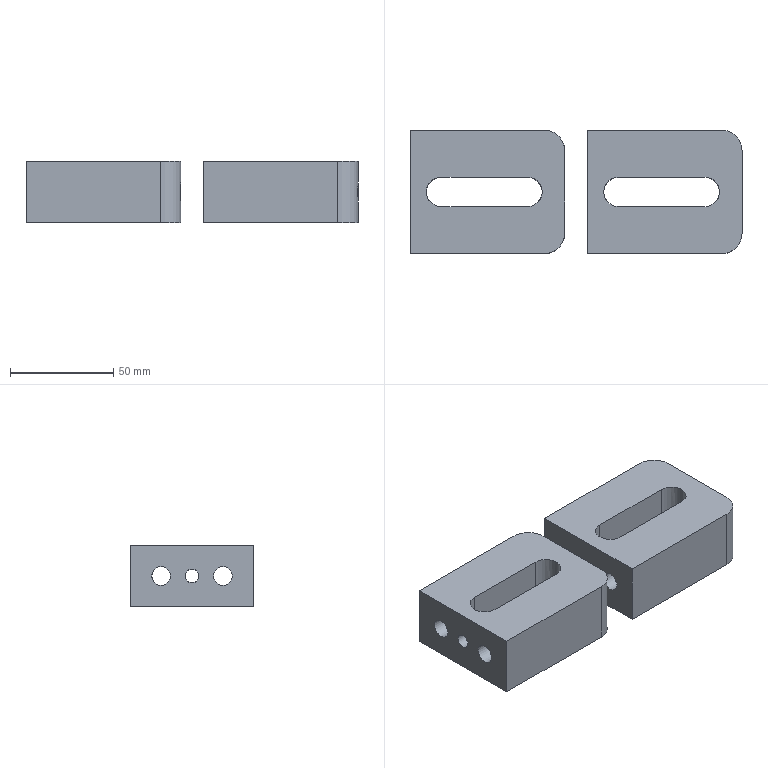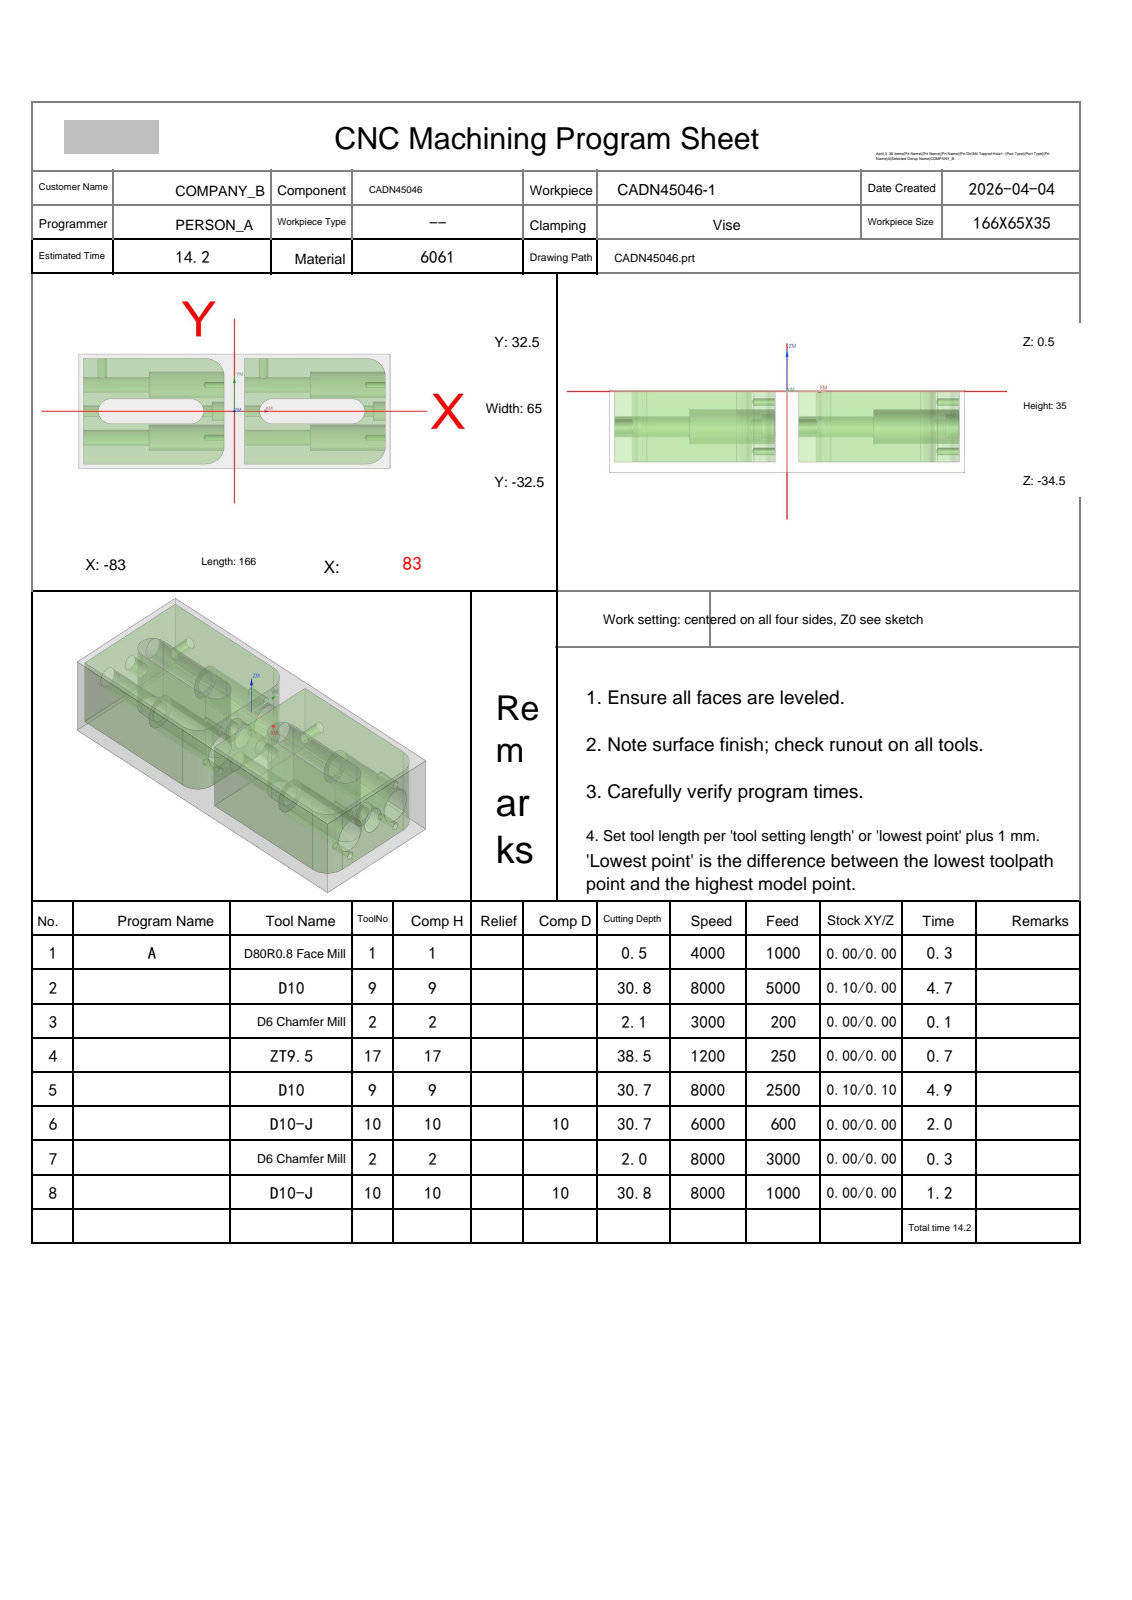NC program | NX | posted by the shop | part box 161 x 60 x 30 mm
Whole program, first 1260 of 1901 lines:
%
O0001
(Machine time: 15.73 MIN)
(===Total Tool:5===)
(T1=D80R0.8 Face Mill D=80.  R=0.8  D-  H01 Z=0.    )
(T9=D10     D=10.  R=0.   D-  H09 Z=-30.3 )
(T2=D6 Chamfer Mill   D=6.   R=0.   D-  H02 Z=-1.55 )
(T17=ZT9.5  D=9.5  DR_a=118 D-  H17 Z=-38.  )
(T10=D10-J  D=10.  R=0.   D10 H10 Z=-30.3 )
G80 G90 G17 G49 G40
G91 G28 Z0
M01
N1 T01 M06
(D80R0.8 Face Mill  D=80. R=0.8 H=01 ce=0.00 di=0.00)
G00 G90 G54 X-125.5 Y0.0 M03 S4000
G43 H01 Z20.
M08
Z2.
G01 Z0.0 F1000.
X-120.5
X120.5
X125.5
Z2.
G00 Z20.
G91 G28 Z0.0
M05
M09
G91 G28 Z0.0
M01
N2 T09 M06
(D10  D=10. R=0. H=09 ce=0.10 di=0.00)
G00 G90 G54 X38. Y35.1 M03 S8000
G43 H09 Z20.
M08
Z.5
G01 X70.5 Z.413 F5000.
G02 X85.6 Y20. Z.349 I0.0 J-15.1
G01 Y-20. Z.241
G02 X70.5 Y-35.1 Z.177 I-15.1 J0.0
G01 X5.5 Z.002
G02 X.4 Y-30. Z-.019 I0.0 J5.1
G01 Y30. Z-.181
G02 X5.5 Y35.1 Z-.202 I5.1 J0.0
G01 X70.5 Z-.377
G02 X85.6 Y20. Z-.441 I0.0 J-15.1
G01 Y-20. Z-.549
G02 X70.5 Y-35.1 Z-.613 I-15.1 J0.0
G01 X5.5 Z-.787
G02 X.4 Y-30. Z-.809 I0.0 J5.1
G01 Y30. Z-.97
G02 X5.5 Y35.1 Z-.992 I5.1 J0.0
G01 X70.5 Z-1.167
G02 X85.6 Y20. Z-1.231 I0.0 J-15.1
G01 Y-20. Z-1.338
G02 X70.5 Y-35.1 Z-1.402 I-15.1 J0.0
G01 X5.5 Z-1.577
G02 X.4 Y-30. Z-1.599 I0.0 J5.1
G01 Y30. Z-1.76
G02 X5.5 Y35.1 Z-1.782 I5.1 J0.0
G01 X70.5 Z-1.957
G02 X85.6 Y20. Z-2.021 I0.0 J-15.1
G01 Y-20. Z-2.128
G02 X70.5 Y-35.1 Z-2.192 I-15.1 J0.0
G01 X5.5 Z-2.367
G02 X.4 Y-30. Z-2.388 I0.0 J5.1
G01 Y30. Z-2.55
G02 X5.5 Y35.1 Z-2.572 I5.1 J0.0
G01 X70.5 Z-2.746
G02 X85.6 Y20. Z-2.81 I0.0 J-15.1
G01 Y-20. Z-2.918
G02 X70.5 Y-35.1 Z-2.982 I-15.1 J0.0
G01 X5.5 Z-3.157
G02 X.4 Y-30. Z-3.178 I0.0 J5.1
G01 Y30. Z-3.34
G02 X5.5 Y35.1 Z-3.361 I5.1 J0.0
G01 X70.5 Z-3.536
G02 X85.6 Y20. Z-3.6 I0.0 J-15.1
G01 Y-20. Z-3.708
G02 X70.5 Y-35.1 Z-3.771 I-15.1 J0.0
G01 X5.5 Z-3.946
G02 X.4 Y-30. Z-3.968 I0.0 J5.1
G01 Y30. Z-4.129
G02 X5.5 Y35.1 Z-4.151 I5.1 J0.0
G01 X70.5 Z-4.326
G02 X85.6 Y20. Z-4.39 I0.0 J-15.1
G01 Y-20. Z-4.497
G02 X70.5 Y-35.1 Z-4.561 I-15.1 J0.0
G01 X5.5 Z-4.736
G02 X.4 Y-30. Z-4.758 I0.0 J5.1
G01 Y30. Z-4.919
G02 X5.5 Y35.1 Z-4.941 I5.1 J0.0
G01 X70.5 Z-5.116
G02 X85.6 Y20. Z-5.179 I0.0 J-15.1
G01 Y-20. Z-5.287
G02 X70.5 Y-35.1 Z-5.351 I-15.1 J0.0
G01 X5.5 Z-5.526
G02 X.4 Y-30. Z-5.547 I0.0 J5.1
G01 Y30. Z-5.709
G02 X5.5 Y35.1 Z-5.73 I5.1 J0.0
G01 X70.5 Z-5.905
G02 X85.6 Y20. Z-5.969 I0.0 J-15.1
G01 Y-20. Z-6.077
G02 X70.5 Y-35.1 Z-6.141 I-15.1 J0.0
G01 X5.5 Z-6.316
G02 X.4 Y-30. Z-6.337 I0.0 J5.1
G01 Y30. Z-6.499
G02 X5.5 Y35.1 Z-6.52 I5.1 J0.0
G01 X70.5 Z-6.695
G02 X85.6 Y20. Z-6.759 I0.0 J-15.1
G01 Y-20. Z-6.867
G02 X70.5 Y-35.1 Z-6.93 I-15.1 J0.0
G01 X5.5 Z-7.105
G02 X.4 Y-30. Z-7.127 I0.0 J5.1
G01 Y30. Z-7.288
G02 X5.5 Y35.1 Z-7.31 I5.1 J0.0
G01 X70.5 Z-7.485
G02 X85.6 Y20. Z-7.549 I0.0 J-15.1
G01 Y-20. Z-7.656
G02 X70.5 Y-35.1 Z-7.72 I-15.1 J0.0
G01 X5.5 Z-7.895
G02 X.4 Y-30. Z-7.917 I0.0 J5.1
G01 Y30. Z-8.078
G02 X5.5 Y35.1 Z-8.1 I5.1 J0.0
G01 X70.5 Z-8.275
G02 X85.6 Y20. Z-8.338 I0.0 J-15.1
G01 Y-20. Z-8.446
G02 X70.5 Y-35.1 Z-8.51 I-15.1 J0.0
G01 X5.5 Z-8.685
G02 X.4 Y-30. Z-8.706 I0.0 J5.1
G01 Y30. Z-8.868
G02 X5.5 Y35.1 Z-8.889 I5.1 J0.0
G01 X70.5 Z-9.064
G02 X85.6 Y20. Z-9.128 I0.0 J-15.1
G01 Y-20. Z-9.236
G02 X70.5 Y-35.1 Z-9.3 I-15.1 J0.0
G01 X5.5 Z-9.475
G02 X.4 Y-30. Z-9.496 I0.0 J5.1
G01 Y30. Z-9.658
G02 X5.5 Y35.1 Z-9.679 I5.1 J0.0
G01 X70.5 Z-9.854
G02 X85.6 Y20. Z-9.918 I0.0 J-15.1
G01 Y-20. Z-10.026
G02 X70.5 Y-35.1 Z-10.089 I-15.1 J0.0
G01 X5.5 Z-10.264
G02 X.4 Y-30. Z-10.286 I0.0 J5.1
G01 Y30. Z-10.447
G02 X5.5 Y35.1 Z-10.469 I5.1 J0.0
G01 X70.5 Z-10.644
G02 X85.6 Y20. Z-10.708 I0.0 J-15.1
G01 Y-20. Z-10.815
G02 X70.5 Y-35.1 Z-10.879 I-15.1 J0.0
G01 X5.5 Z-11.054
G02 X.4 Y-30. Z-11.076 I0.0 J5.1
G01 Y30. Z-11.237
G02 X5.5 Y35.1 Z-11.259 I5.1 J0.0
G01 X70.5 Z-11.434
G02 X85.6 Y20. Z-11.497 I0.0 J-15.1
G01 Y-20. Z-11.605
G02 X70.5 Y-35.1 Z-11.669 I-15.1 J0.0
G01 X5.5 Z-11.844
G02 X.4 Y-30. Z-11.865 I0.0 J5.1
G01 Y30. Z-12.027
G02 X5.5 Y35.1 Z-12.048 I5.1 J0.0
G01 X70.5 Z-12.223
G02 X85.6 Y20. Z-12.287 I0.0 J-15.1
G01 Y-20. Z-12.395
G02 X70.5 Y-35.1 Z-12.459 I-15.1 J0.0
G01 X5.5 Z-12.634
G02 X.4 Y-30. Z-12.655 I0.0 J5.1
G01 Y30. Z-12.817
G02 X5.5 Y35.1 Z-12.838 I5.1 J0.0
G01 X70.5 Z-13.013
G02 X85.6 Y20. Z-13.077 I0.0 J-15.1
G01 Y-20. Z-13.185
G02 X70.5 Y-35.1 Z-13.248 I-15.1 J0.0
G01 X5.5 Z-13.423
G02 X.4 Y-30. Z-13.445 I0.0 J5.1
G01 Y30. Z-13.606
G02 X5.5 Y35.1 Z-13.628 I5.1 J0.0
G01 X70.5 Z-13.803
G02 X85.6 Y20. Z-13.867 I0.0 J-15.1
G01 Y-20. Z-13.974
G02 X70.5 Y-35.1 Z-14.038 I-15.1 J0.0
G01 X5.5 Z-14.213
G02 X.4 Y-30. Z-14.235 I0.0 J5.1
G01 Y30. Z-14.396
G02 X5.5 Y35.1 Z-14.418 I5.1 J0.0
G01 X70.5 Z-14.593
G02 X85.6 Y20. Z-14.656 I0.0 J-15.1
G01 Y-20. Z-14.764
G02 X70.5 Y-35.1 Z-14.828 I-15.1 J0.0
G01 X5.5 Z-15.003
G02 X.4 Y-30. Z-15.024 I0.0 J5.1
G01 Y30. Z-15.186
G02 X5.5 Y35.1 Z-15.207 I5.1 J0.0
G01 X70.5 Z-15.382
G02 X85.6 Y20. Z-15.446 I0.0 J-15.1
G01 Y-20. Z-15.554
G02 X70.5 Y-35.1 Z-15.618 I-15.1 J0.0
G01 X5.5 Z-15.793
G02 X.4 Y-30. Z-15.814 I0.0 J5.1
G01 Y30. Z-15.976
G02 X5.5 Y35.1 Z-15.997 I5.1 J0.0
G01 X70.5 Z-16.172
G02 X85.6 Y20. Z-16.236 I0.0 J-15.1
G01 Y-20. Z-16.344
G02 X70.5 Y-35.1 Z-16.407 I-15.1 J0.0
G01 X5.5 Z-16.582
G02 X.4 Y-30. Z-16.604 I0.0 J5.1
G01 Y30. Z-16.765
G02 X5.5 Y35.1 Z-16.787 I5.1 J0.0
G01 X70.5 Z-16.962
G02 X85.6 Y20. Z-17.026 I0.0 J-15.1
G01 Y-20. Z-17.133
G02 X70.5 Y-35.1 Z-17.197 I-15.1 J0.0
G01 X5.5 Z-17.372
G02 X.4 Y-30. Z-17.394 I0.0 J5.1
G01 Y30. Z-17.555
G02 X5.5 Y35.1 Z-17.577 I5.1 J0.0
G01 X70.5 Z-17.752
G02 X85.6 Y20. Z-17.815 I0.0 J-15.1
G01 Y-20. Z-17.923
G02 X70.5 Y-35.1 Z-17.987 I-15.1 J0.0
G01 X5.5 Z-18.162
G02 X.4 Y-30. Z-18.183 I0.0 J5.1
G01 Y30. Z-18.345
G02 X5.5 Y35.1 Z-18.366 I5.1 J0.0
G01 X70.5 Z-18.541
G02 X85.6 Y20. Z-18.605 I0.0 J-15.1
G01 Y-20. Z-18.713
G02 X70.5 Y-35.1 Z-18.777 I-15.1 J0.0
G01 X5.5 Z-18.952
G02 X.4 Y-30. Z-18.973 I0.0 J5.1
G01 Y30. Z-19.135
G02 X5.5 Y35.1 Z-19.156 I5.1 J0.0
G01 X70.5 Z-19.331
G02 X85.6 Y20. Z-19.395 I0.0 J-15.1
G01 Y-20. Z-19.503
G02 X70.5 Y-35.1 Z-19.566 I-15.1 J0.0
G01 X5.5 Z-19.741
G02 X.4 Y-30. Z-19.763 I0.0 J5.1
G01 Y30. Z-19.924
G02 X5.5 Y35.1 Z-19.946 I5.1 J0.0
G01 X70.5 Z-20.121
G02 X85.6 Y20. Z-20.185 I0.0 J-15.1
G01 Y-20. Z-20.292
G02 X70.5 Y-35.1 Z-20.356 I-15.1 J0.0
G01 X5.5 Z-20.531
G02 X.4 Y-30. Z-20.553 I0.0 J5.1
G01 Y30. Z-20.714
G02 X5.5 Y35.1 Z-20.736 I5.1 J0.0
G01 X70.5 Z-20.911
G02 X85.6 Y20. Z-20.974 I0.0 J-15.1
G01 Y-20. Z-21.082
G02 X70.5 Y-35.1 Z-21.146 I-15.1 J0.0
G01 X5.5 Z-21.321
G02 X.4 Y-30. Z-21.342 I0.0 J5.1
G01 Y30. Z-21.504
G02 X5.5 Y35.1 Z-21.525 I5.1 J0.0
G01 X70.5 Z-21.7
G02 X85.6 Y20. Z-21.764 I0.0 J-15.1
G01 Y-20. Z-21.872
G02 X70.5 Y-35.1 Z-21.936 I-15.1 J0.0
G01 X5.5 Z-22.111
G02 X.4 Y-30. Z-22.132 I0.0 J5.1
G01 Y30. Z-22.294
G02 X5.5 Y35.1 Z-22.315 I5.1 J0.0
G01 X70.5 Z-22.49
G02 X85.6 Y20. Z-22.554 I0.0 J-15.1
G01 Y-20. Z-22.662
G02 X70.5 Y-35.1 Z-22.725 I-15.1 J0.0
G01 X5.5 Z-22.9
G02 X.4 Y-30. Z-22.922 I0.0 J5.1
G01 Y30. Z-23.083
G02 X5.5 Y35.1 Z-23.105 I5.1 J0.0
G01 X70.5 Z-23.28
G02 X85.6 Y20. Z-23.344 I0.0 J-15.1
G01 Y-20. Z-23.451
G02 X70.5 Y-35.1 Z-23.515 I-15.1 J0.0
G01 X5.5 Z-23.69
G02 X.4 Y-30. Z-23.712 I0.0 J5.1
G01 Y30. Z-23.873
G02 X5.5 Y35.1 Z-23.895 I5.1 J0.0
G01 X70.5 Z-24.07
G02 X85.6 Y20. Z-24.133 I0.0 J-15.1
G01 Y-20. Z-24.241
G02 X70.5 Y-35.1 Z-24.305 I-15.1 J0.0
G01 X5.5 Z-24.48
G02 X.4 Y-30. Z-24.501 I0.0 J5.1
G01 Y30. Z-24.663
G02 X5.5 Y35.1 Z-24.684 I5.1 J0.0
G01 X70.5 Z-24.859
G02 X85.6 Y20. Z-24.923 I0.0 J-15.1
G01 Y-20. Z-25.031
G02 X70.5 Y-35.1 Z-25.095 I-15.1 J0.0
G01 X5.5 Z-25.269
G02 X.4 Y-30. Z-25.291 I0.0 J5.1
G01 Y30. Z-25.453
G02 X5.5 Y35.1 Z-25.474 I5.1 J0.0
G01 X70.5 Z-25.649
G02 X85.6 Y20. Z-25.713 I0.0 J-15.1
G01 Y-20. Z-25.82
G02 X70.5 Y-35.1 Z-25.884 I-15.1 J0.0
G01 X5.5 Z-26.059
G02 X.4 Y-30. Z-26.081 I0.0 J5.1
G01 Y30. Z-26.242
G02 X5.5 Y35.1 Z-26.264 I5.1 J0.0
G01 X70.5 Z-26.439
G02 X85.6 Y20. Z-26.503 I0.0 J-15.1
G01 Y-20. Z-26.61
G02 X70.5 Y-35.1 Z-26.674 I-15.1 J0.0
G01 X5.5 Z-26.849
G02 X.4 Y-30. Z-26.871 I0.0 J5.1
G01 Y30. Z-27.032
G02 X5.5 Y35.1 Z-27.054 I5.1 J0.0
G01 X70.5 Z-27.228
G02 X85.6 Y20. Z-27.292 I0.0 J-15.1
G01 Y-20. Z-27.4
G02 X70.5 Y-35.1 Z-27.464 I-15.1 J0.0
G01 X5.5 Z-27.639
G02 X.4 Y-30. Z-27.66 I0.0 J5.1
G01 Y30. Z-27.822
G02 X5.5 Y35.1 Z-27.843 I5.1 J0.0
G01 X70.5 Z-28.018
G02 X85.6 Y20. Z-28.082 I0.0 J-15.1
G01 Y-20. Z-28.19
G02 X70.5 Y-35.1 Z-28.254 I-15.1 J0.0
G01 X5.5 Z-28.428
G02 X.4 Y-30. Z-28.45 I0.0 J5.1
G01 Y30. Z-28.611
G02 X5.5 Y35.1 Z-28.633 I5.1 J0.0
G01 X70.5 Z-28.808
G02 X85.6 Y20. Z-28.872 I0.0 J-15.1
G01 Y-20. Z-28.979
G02 X70.5 Y-35.1 Z-29.043 I-15.1 J0.0
G01 X5.5 Z-29.218
G02 X.4 Y-30. Z-29.24 I0.0 J5.1
G01 Y30. Z-29.401
G02 X5.5 Y35.1 Z-29.423 I5.1 J0.0
G01 X70.5 Z-29.598
G02 X85.6 Y20. Z-29.662 I0.0 J-15.1
G01 Y-20. Z-29.769
G02 X70.5 Y-35.1 Z-29.833 I-15.1 J0.0
G01 X5.5 Z-30.008
G02 X.4 Y-30. Z-30.03 I0.0 J5.1
G01 Y30. Z-30.191
G02 X5.5 Y35.1 Z-30.213 I5.1 J0.0
G01 X38. Z-30.3
X70.5
G02 X85.6 Y20. I0.0 J-15.1
G01 Y-20.
G02 X70.5 Y-35.1 I-15.1 J0.0
G01 X5.5
G02 X.4 Y-30. I0.0 J5.1
G01 Y30.
G02 X5.5 Y35.1 I5.1 J0.0
G01 X38.
X38.5
Z-29.3
G00 Z20.
X-48.
Z.5
G01 X-15.5 Z.413
G02 X-.4 Y20. Z.349 I0.0 J-15.1
G01 Y-20. Z.241
G02 X-15.5 Y-35.1 Z.177 I-15.1 J0.0
G01 X-80.5 Z.002
G02 X-85.6 Y-30. Z-.019 I0.0 J5.1
G01 Y30. Z-.181
G02 X-80.5 Y35.1 Z-.202 I5.1 J0.0
G01 X-15.5 Z-.377
G02 X-.4 Y20. Z-.441 I0.0 J-15.1
G01 Y-20. Z-.549
G02 X-15.5 Y-35.1 Z-.613 I-15.1 J0.0
G01 X-80.5 Z-.787
G02 X-85.6 Y-30. Z-.809 I0.0 J5.1
G01 Y30. Z-.97
G02 X-80.5 Y35.1 Z-.992 I5.1 J0.0
G01 X-15.5 Z-1.167
G02 X-.4 Y20. Z-1.231 I0.0 J-15.1
G01 Y-20. Z-1.338
G02 X-15.5 Y-35.1 Z-1.402 I-15.1 J0.0
G01 X-80.5 Z-1.577
G02 X-85.6 Y-30. Z-1.599 I0.0 J5.1
G01 Y30. Z-1.76
G02 X-80.5 Y35.1 Z-1.782 I5.1 J0.0
G01 X-15.5 Z-1.957
G02 X-.4 Y20. Z-2.021 I0.0 J-15.1
G01 Y-20. Z-2.128
G02 X-15.5 Y-35.1 Z-2.192 I-15.1 J0.0
G01 X-80.5 Z-2.367
G02 X-85.6 Y-30. Z-2.388 I0.0 J5.1
G01 Y30. Z-2.55
G02 X-80.5 Y35.1 Z-2.572 I5.1 J0.0
G01 X-15.5 Z-2.746
G02 X-.4 Y20. Z-2.81 I0.0 J-15.1
G01 Y-20. Z-2.918
G02 X-15.5 Y-35.1 Z-2.982 I-15.1 J0.0
G01 X-80.5 Z-3.157
G02 X-85.6 Y-30. Z-3.178 I0.0 J5.1
G01 Y30. Z-3.34
G02 X-80.5 Y35.1 Z-3.361 I5.1 J0.0
G01 X-15.5 Z-3.536
G02 X-.4 Y20. Z-3.6 I0.0 J-15.1
G01 Y-20. Z-3.708
G02 X-15.5 Y-35.1 Z-3.771 I-15.1 J0.0
G01 X-80.5 Z-3.946
G02 X-85.6 Y-30. Z-3.968 I0.0 J5.1
G01 Y30. Z-4.129
G02 X-80.5 Y35.1 Z-4.151 I5.1 J0.0
G01 X-15.5 Z-4.326
G02 X-.4 Y20. Z-4.39 I0.0 J-15.1
G01 Y-20. Z-4.497
G02 X-15.5 Y-35.1 Z-4.561 I-15.1 J0.0
G01 X-80.5 Z-4.736
G02 X-85.6 Y-30. Z-4.758 I0.0 J5.1
G01 Y30. Z-4.919
G02 X-80.5 Y35.1 Z-4.941 I5.1 J0.0
G01 X-15.5 Z-5.116
G02 X-.4 Y20. Z-5.179 I0.0 J-15.1
G01 Y-20. Z-5.287
G02 X-15.5 Y-35.1 Z-5.351 I-15.1 J0.0
G01 X-80.5 Z-5.526
G02 X-85.6 Y-30. Z-5.547 I0.0 J5.1
G01 Y30. Z-5.709
G02 X-80.5 Y35.1 Z-5.73 I5.1 J0.0
G01 X-15.5 Z-5.905
G02 X-.4 Y20. Z-5.969 I0.0 J-15.1
G01 Y-20. Z-6.077
G02 X-15.5 Y-35.1 Z-6.141 I-15.1 J0.0
G01 X-80.5 Z-6.316
G02 X-85.6 Y-30. Z-6.337 I0.0 J5.1
G01 Y30. Z-6.499
G02 X-80.5 Y35.1 Z-6.52 I5.1 J0.0
G01 X-15.5 Z-6.695
G02 X-.4 Y20. Z-6.759 I0.0 J-15.1
G01 Y-20. Z-6.867
G02 X-15.5 Y-35.1 Z-6.93 I-15.1 J0.0
G01 X-80.5 Z-7.105
G02 X-85.6 Y-30. Z-7.127 I0.0 J5.1
G01 Y30. Z-7.288
G02 X-80.5 Y35.1 Z-7.31 I5.1 J0.0
G01 X-15.5 Z-7.485
G02 X-.4 Y20. Z-7.549 I0.0 J-15.1
G01 Y-20. Z-7.656
G02 X-15.5 Y-35.1 Z-7.72 I-15.1 J0.0
G01 X-80.5 Z-7.895
G02 X-85.6 Y-30. Z-7.917 I0.0 J5.1
G01 Y30. Z-8.078
G02 X-80.5 Y35.1 Z-8.1 I5.1 J0.0
G01 X-15.5 Z-8.275
G02 X-.4 Y20. Z-8.338 I0.0 J-15.1
G01 Y-20. Z-8.446
G02 X-15.5 Y-35.1 Z-8.51 I-15.1 J0.0
G01 X-80.5 Z-8.685
G02 X-85.6 Y-30. Z-8.706 I0.0 J5.1
G01 Y30. Z-8.868
G02 X-80.5 Y35.1 Z-8.889 I5.1 J0.0
G01 X-15.5 Z-9.064
G02 X-.4 Y20. Z-9.128 I0.0 J-15.1
G01 Y-20. Z-9.236
G02 X-15.5 Y-35.1 Z-9.3 I-15.1 J0.0
G01 X-80.5 Z-9.475
G02 X-85.6 Y-30. Z-9.496 I0.0 J5.1
G01 Y30. Z-9.658
G02 X-80.5 Y35.1 Z-9.679 I5.1 J0.0
G01 X-15.5 Z-9.854
G02 X-.4 Y20. Z-9.918 I0.0 J-15.1
G01 Y-20. Z-10.026
G02 X-15.5 Y-35.1 Z-10.089 I-15.1 J0.0
G01 X-80.5 Z-10.264
G02 X-85.6 Y-30. Z-10.286 I0.0 J5.1
G01 Y30. Z-10.447
G02 X-80.5 Y35.1 Z-10.469 I5.1 J0.0
G01 X-15.5 Z-10.644
G02 X-.4 Y20. Z-10.708 I0.0 J-15.1
G01 Y-20. Z-10.815
G02 X-15.5 Y-35.1 Z-10.879 I-15.1 J0.0
G01 X-80.5 Z-11.054
G02 X-85.6 Y-30. Z-11.076 I0.0 J5.1
G01 Y30. Z-11.237
G02 X-80.5 Y35.1 Z-11.259 I5.1 J0.0
G01 X-15.5 Z-11.434
G02 X-.4 Y20. Z-11.497 I0.0 J-15.1
G01 Y-20. Z-11.605
G02 X-15.5 Y-35.1 Z-11.669 I-15.1 J0.0
G01 X-80.5 Z-11.844
G02 X-85.6 Y-30. Z-11.865 I0.0 J5.1
G01 Y30. Z-12.027
G02 X-80.5 Y35.1 Z-12.048 I5.1 J0.0
G01 X-15.5 Z-12.223
G02 X-.4 Y20. Z-12.287 I0.0 J-15.1
G01 Y-20. Z-12.395
G02 X-15.5 Y-35.1 Z-12.459 I-15.1 J0.0
G01 X-80.5 Z-12.634
G02 X-85.6 Y-30. Z-12.655 I0.0 J5.1
G01 Y30. Z-12.817
G02 X-80.5 Y35.1 Z-12.838 I5.1 J0.0
G01 X-15.5 Z-13.013
G02 X-.4 Y20. Z-13.077 I0.0 J-15.1
G01 Y-20. Z-13.185
G02 X-15.5 Y-35.1 Z-13.248 I-15.1 J0.0
G01 X-80.5 Z-13.423
G02 X-85.6 Y-30. Z-13.445 I0.0 J5.1
G01 Y30. Z-13.606
G02 X-80.5 Y35.1 Z-13.628 I5.1 J0.0
G01 X-15.5 Z-13.803
G02 X-.4 Y20. Z-13.867 I0.0 J-15.1
G01 Y-20. Z-13.974
G02 X-15.5 Y-35.1 Z-14.038 I-15.1 J0.0
G01 X-80.5 Z-14.213
G02 X-85.6 Y-30. Z-14.235 I0.0 J5.1
G01 Y30. Z-14.396
G02 X-80.5 Y35.1 Z-14.418 I5.1 J0.0
G01 X-15.5 Z-14.593
G02 X-.4 Y20. Z-14.656 I0.0 J-15.1
G01 Y-20. Z-14.764
G02 X-15.5 Y-35.1 Z-14.828 I-15.1 J0.0
G01 X-80.5 Z-15.003
G02 X-85.6 Y-30. Z-15.024 I0.0 J5.1
G01 Y30. Z-15.186
G02 X-80.5 Y35.1 Z-15.207 I5.1 J0.0
G01 X-15.5 Z-15.382
G02 X-.4 Y20. Z-15.446 I0.0 J-15.1
G01 Y-20. Z-15.554
G02 X-15.5 Y-35.1 Z-15.618 I-15.1 J0.0
G01 X-80.5 Z-15.793
G02 X-85.6 Y-30. Z-15.814 I0.0 J5.1
G01 Y30. Z-15.976
G02 X-80.5 Y35.1 Z-15.997 I5.1 J0.0
G01 X-15.5 Z-16.172
G02 X-.4 Y20. Z-16.236 I0.0 J-15.1
G01 Y-20. Z-16.344
G02 X-15.5 Y-35.1 Z-16.407 I-15.1 J0.0
G01 X-80.5 Z-16.582
G02 X-85.6 Y-30. Z-16.604 I0.0 J5.1
G01 Y30. Z-16.765
G02 X-80.5 Y35.1 Z-16.787 I5.1 J0.0
G01 X-15.5 Z-16.962
G02 X-.4 Y20. Z-17.026 I0.0 J-15.1
G01 Y-20. Z-17.133
G02 X-15.5 Y-35.1 Z-17.197 I-15.1 J0.0
G01 X-80.5 Z-17.372
G02 X-85.6 Y-30. Z-17.394 I0.0 J5.1
G01 Y30. Z-17.555
G02 X-80.5 Y35.1 Z-17.577 I5.1 J0.0
G01 X-15.5 Z-17.752
G02 X-.4 Y20. Z-17.815 I0.0 J-15.1
G01 Y-20. Z-17.923
G02 X-15.5 Y-35.1 Z-17.987 I-15.1 J0.0
G01 X-80.5 Z-18.162
G02 X-85.6 Y-30. Z-18.183 I0.0 J5.1
G01 Y30. Z-18.345
G02 X-80.5 Y35.1 Z-18.366 I5.1 J0.0
G01 X-15.5 Z-18.541
G02 X-.4 Y20. Z-18.605 I0.0 J-15.1
G01 Y-20. Z-18.713
G02 X-15.5 Y-35.1 Z-18.777 I-15.1 J0.0
G01 X-80.5 Z-18.952
G02 X-85.6 Y-30. Z-18.973 I0.0 J5.1
G01 Y30. Z-19.135
G02 X-80.5 Y35.1 Z-19.156 I5.1 J0.0
G01 X-15.5 Z-19.331
G02 X-.4 Y20. Z-19.395 I0.0 J-15.1
G01 Y-20. Z-19.503
G02 X-15.5 Y-35.1 Z-19.566 I-15.1 J0.0
G01 X-80.5 Z-19.741
G02 X-85.6 Y-30. Z-19.763 I0.0 J5.1
G01 Y30. Z-19.924
G02 X-80.5 Y35.1 Z-19.946 I5.1 J0.0
G01 X-15.5 Z-20.121
G02 X-.4 Y20. Z-20.185 I0.0 J-15.1
G01 Y-20. Z-20.292
G02 X-15.5 Y-35.1 Z-20.356 I-15.1 J0.0
G01 X-80.5 Z-20.531
G02 X-85.6 Y-30. Z-20.553 I0.0 J5.1
G01 Y30. Z-20.714
G02 X-80.5 Y35.1 Z-20.736 I5.1 J0.0
G01 X-15.5 Z-20.911
G02 X-.4 Y20. Z-20.974 I0.0 J-15.1
G01 Y-20. Z-21.082
G02 X-15.5 Y-35.1 Z-21.146 I-15.1 J0.0
G01 X-80.5 Z-21.321
G02 X-85.6 Y-30. Z-21.342 I0.0 J5.1
G01 Y30. Z-21.504
G02 X-80.5 Y35.1 Z-21.525 I5.1 J0.0
G01 X-15.5 Z-21.7
G02 X-.4 Y20. Z-21.764 I0.0 J-15.1
G01 Y-20. Z-21.872
G02 X-15.5 Y-35.1 Z-21.936 I-15.1 J0.0
G01 X-80.5 Z-22.111
G02 X-85.6 Y-30. Z-22.132 I0.0 J5.1
G01 Y30. Z-22.294
G02 X-80.5 Y35.1 Z-22.315 I5.1 J0.0
G01 X-15.5 Z-22.49
G02 X-.4 Y20. Z-22.554 I0.0 J-15.1
G01 Y-20. Z-22.662
G02 X-15.5 Y-35.1 Z-22.725 I-15.1 J0.0
G01 X-80.5 Z-22.9
G02 X-85.6 Y-30. Z-22.922 I0.0 J5.1
G01 Y30. Z-23.083
G02 X-80.5 Y35.1 Z-23.105 I5.1 J0.0
G01 X-15.5 Z-23.28
G02 X-.4 Y20. Z-23.344 I0.0 J-15.1
G01 Y-20. Z-23.451
G02 X-15.5 Y-35.1 Z-23.515 I-15.1 J0.0
G01 X-80.5 Z-23.69
G02 X-85.6 Y-30. Z-23.712 I0.0 J5.1
G01 Y30. Z-23.873
G02 X-80.5 Y35.1 Z-23.895 I5.1 J0.0
G01 X-15.5 Z-24.07
G02 X-.4 Y20. Z-24.133 I0.0 J-15.1
G01 Y-20. Z-24.241
G02 X-15.5 Y-35.1 Z-24.305 I-15.1 J0.0
G01 X-80.5 Z-24.48
G02 X-85.6 Y-30. Z-24.501 I0.0 J5.1
G01 Y30. Z-24.663
G02 X-80.5 Y35.1 Z-24.684 I5.1 J0.0
G01 X-15.5 Z-24.859
G02 X-.4 Y20. Z-24.923 I0.0 J-15.1
G01 Y-20. Z-25.031
G02 X-15.5 Y-35.1 Z-25.095 I-15.1 J0.0
G01 X-80.5 Z-25.269
G02 X-85.6 Y-30. Z-25.291 I0.0 J5.1
G01 Y30. Z-25.453
G02 X-80.5 Y35.1 Z-25.474 I5.1 J0.0
G01 X-15.5 Z-25.649
G02 X-.4 Y20. Z-25.713 I0.0 J-15.1
G01 Y-20. Z-25.82
G02 X-15.5 Y-35.1 Z-25.884 I-15.1 J0.0
G01 X-80.5 Z-26.059
G02 X-85.6 Y-30. Z-26.081 I0.0 J5.1
G01 Y30. Z-26.242
G02 X-80.5 Y35.1 Z-26.264 I5.1 J0.0
G01 X-15.5 Z-26.439
G02 X-.4 Y20. Z-26.503 I0.0 J-15.1
G01 Y-20. Z-26.61
G02 X-15.5 Y-35.1 Z-26.674 I-15.1 J0.0
G01 X-80.5 Z-26.849
G02 X-85.6 Y-30. Z-26.871 I0.0 J5.1
G01 Y30. Z-27.032
G02 X-80.5 Y35.1 Z-27.054 I5.1 J0.0
G01 X-15.5 Z-27.228
G02 X-.4 Y20. Z-27.292 I0.0 J-15.1
G01 Y-20. Z-27.4
G02 X-15.5 Y-35.1 Z-27.464 I-15.1 J0.0
G01 X-80.5 Z-27.639
G02 X-85.6 Y-30. Z-27.66 I0.0 J5.1
G01 Y30. Z-27.822
G02 X-80.5 Y35.1 Z-27.843 I5.1 J0.0
G01 X-15.5 Z-28.018
G02 X-.4 Y20. Z-28.082 I0.0 J-15.1
G01 Y-20. Z-28.19
G02 X-15.5 Y-35.1 Z-28.254 I-15.1 J0.0
G01 X-80.5 Z-28.428
G02 X-85.6 Y-30. Z-28.45 I0.0 J5.1
G01 Y30. Z-28.611
G02 X-80.5 Y35.1 Z-28.633 I5.1 J0.0
G01 X-15.5 Z-28.808
G02 X-.4 Y20. Z-28.872 I0.0 J-15.1
G01 Y-20. Z-28.979
G02 X-15.5 Y-35.1 Z-29.043 I-15.1 J0.0
G01 X-80.5 Z-29.218
G02 X-85.6 Y-30. Z-29.24 I0.0 J5.1
G01 Y30. Z-29.401
G02 X-80.5 Y35.1 Z-29.423 I5.1 J0.0
G01 X-15.5 Z-29.598
G02 X-.4 Y20. Z-29.662 I0.0 J-15.1
G01 Y-20. Z-29.769
G02 X-15.5 Y-35.1 Z-29.833 I-15.1 J0.0
G01 X-80.5 Z-30.008
G02 X-85.6 Y-30. Z-30.03 I0.0 J5.1
G01 Y30. Z-30.191
G02 X-80.5 Y35.1 Z-30.213 I5.1 J0.0
G01 X-48. Z-30.3
X-15.5
G02 X-.4 Y20. I0.0 J-15.1
G01 Y-20.
G02 X-15.5 Y-35.1 I-15.1 J0.0
G01 X-80.5
G02 X-85.6 Y-30. I0.0 J5.1
G01 Y30.
G02 X-80.5 Y35.1 I5.1 J0.0
G01 X-48.
X-47.5
Z-29.3
G00 Z20.
G91 G28 Z0.0
M05
M09
G91 G28 Z0.0
M01
N3 T02 M06
(D6 Chamfer Mill  D=6. R=0. H=02 ce=0.00 di=0.00)
G00 G90 G54 X-65.5 Y0.0 M03 S3000
G43 H02 Z20.
M08
G98 G81 X-65.5 Y0.0 Z-1.55 R1. F200.
X-23.5
X20.5
X62.5
G80
G00 Z20.
G91 G28 Z0.0
M05
M09
G91 G28 Z0.0
M01
N4 T17 M06
(ZT9.5 D=9.5 DR_a=118 H=17)
G00 G90 G54 X-65.5 Y0.0 M03 S1200
G43 H17 Z20.
M08
G98 G83 X-65.5 Y0.0 Z-38. R1. F250. Q3.
X-23.5
X20.5
X62.5
G80
G00 Z20.
G91 G28 Z0.0
M05
M09
G91 G28 Z0.0
M01
N5 T09 M06
(D10  D=10. R=0. H=09 ce=0.10 di=0.10)
G00 G90 G54 X-44.5 Y-2. M03 S8000
G43 H09 Z20.
M08
Z.5
G01 X-23.5 Z.392 F2500.
G03 X-21.5 Y0.0 Z.376 I0.0 J2.
X-23.5 Y2. Z.36 I-2. J0.0
G01 X-65.5 Z.145
G03 X-67.5 Y0.0 Z.129 I0.0 J-2.
X-65.5 Y-2. Z.113 I2. J0.0
G01 X-23.5 Z-.103
G03 X-21.5 Y0.0 Z-.119 I0.0 J2.
X-23.5 Y2. Z-.135 I-2. J0.0
G01 X-65.5 Z-.35
G03 X-67.5 Y0.0 Z-.367 I0.0 J-2.
X-65.5 Y-2. Z-.383 I2. J0.0
G01 X-23.5 Z-.598
G03 X-21.5 Y0.0 Z-.614 I0.0 J2.
X-23.5 Y2. Z-.63 I-2. J0.0
G01 X-65.5 Z-.846
G03 X-67.5 Y0.0 Z-.862 I0.0 J-2.
X-65.5 Y-2. Z-.878 I2. J0.0
G01 X-23.5 Z-1.093
G03 X-21.5 Y0.0 Z-1.109 I0.0 J2.
X-23.5 Y2. Z-1.125 I-2. J0.0
G01 X-65.5 Z-1.341
G03 X-67.5 Y0.0 Z-1.357 I0.0 J-2.
X-65.5 Y-2. Z-1.373 I2. J0.0
G01 X-23.5 Z-1.588
G03 X-21.5 Y0.0 Z-1.604 I0.0 J2.
X-23.5 Y2. Z-1.621 I-2. J0.0
G01 X-65.5 Z-1.836
G03 X-67.5 Y0.0 Z-1.852 I0.0 J-2.
X-65.5 Y-2. Z-1.868 I2. J0.0
G01 X-23.5 Z-2.083
G03 X-21.5 Y0.0 Z-2.1 I0.0 J2.
X-23.5 Y2. Z-2.116 I-2. J0.0
G01 X-65.5 Z-2.331
G03 X-67.5 Y0.0 Z-2.347 I0.0 J-2.
X-65.5 Y-2. Z-2.363 I2. J0.0
G01 X-23.5 Z-2.579
G03 X-21.5 Y0.0 Z-2.595 I0.0 J2.
X-23.5 Y2. Z-2.611 I-2. J0.0
G01 X-65.5 Z-2.826
G03 X-67.5 Y0.0 Z-2.842 I0.0 J-2.
X-65.5 Y-2. Z-2.858 I2. J0.0
G01 X-23.5 Z-3.074
G03 X-21.5 Y0.0 Z-3.09 I0.0 J2.
X-23.5 Y2. Z-3.106 I-2. J0.0
G01 X-65.5 Z-3.321
G03 X-67.5 Y0.0 Z-3.338 I0.0 J-2.
X-65.5 Y-2. Z-3.354 I2. J0.0
G01 X-23.5 Z-3.569
G03 X-21.5 Y0.0 Z-3.585 I0.0 J2.
X-23.5 Y2. Z-3.601 I-2. J0.0
G01 X-65.5 Z-3.817
G03 X-67.5 Y0.0 Z-3.833 I0.0 J-2.
X-65.5 Y-2. Z-3.849 I2. J0.0
G01 X-23.5 Z-4.064
G03 X-21.5 Y0.0 Z-4.08 I0.0 J2.
X-23.5 Y2. Z-4.096 I-2. J0.0
G01 X-65.5 Z-4.312
G03 X-67.5 Y0.0 Z-4.328 I0.0 J-2.
X-65.5 Y-2. Z-4.344 I2. J0.0
G01 X-23.5 Z-4.559
G03 X-21.5 Y0.0 Z-4.575 I0.0 J2.
X-23.5 Y2. Z-4.592 I-2. J0.0
G01 X-65.5 Z-4.807
G03 X-67.5 Y0.0 Z-4.823 I0.0 J-2.
X-65.5 Y-2. Z-4.839 I2. J0.0
G01 X-23.5 Z-5.054
G03 X-21.5 Y0.0 Z-5.071 I0.0 J2.
X-23.5 Y2. Z-5.087 I-2. J0.0
G01 X-65.5 Z-5.302
G03 X-67.5 Y0.0 Z-5.318 I0.0 J-2.
X-65.5 Y-2. Z-5.334 I2. J0.0
G01 X-23.5 Z-5.55
G03 X-21.5 Y0.0 Z-5.566 I0.0 J2.
X-23.5 Y2. Z-5.582 I-2. J0.0
G01 X-65.5 Z-5.797
G03 X-67.5 Y0.0 Z-5.813 I0.0 J-2.
X-65.5 Y-2. Z-5.829 I2. J0.0
G01 X-23.5 Z-6.045
G03 X-21.5 Y0.0 Z-6.061 I0.0 J2.
X-23.5 Y2. Z-6.077 I-2. J0.0
G01 X-65.5 Z-6.292
G03 X-67.5 Y0.0 Z-6.308 I0.0 J-2.
X-65.5 Y-2. Z-6.325 I2. J0.0
G01 X-23.5 Z-6.54
G03 X-21.5 Y0.0 Z-6.556 I0.0 J2.
X-23.5 Y2. Z-6.572 I-2. J0.0
G01 X-65.5 Z-6.788
G03 X-67.5 Y0.0 Z-6.804 I0.0 J-2.
X-65.5 Y-2. Z-6.82 I2. J0.0
G01 X-23.5 Z-7.035
G03 X-21.5 Y0.0 Z-7.051 I0.0 J2.
X-23.5 Y2. Z-7.067 I-2. J0.0
G01 X-65.5 Z-7.283
G03 X-67.5 Y0.0 Z-7.299 I0.0 J-2.
X-65.5 Y-2. Z-7.315 I2. J0.0
G01 X-23.5 Z-7.53
G03 X-21.5 Y0.0 Z-7.546 I0.0 J2.
X-23.5 Y2. Z-7.562 I-2. J0.0
G01 X-65.5 Z-7.778
G03 X-67.5 Y0.0 Z-7.794 I0.0 J-2.
X-65.5 Y-2. Z-7.81 I2. J0.0
G01 X-23.5 Z-8.025
G03 X-21.5 Y0.0 Z-8.042 I0.0 J2.
X-23.5 Y2. Z-8.058 I-2. J0.0
G01 X-65.5 Z-8.273
G03 X-67.5 Y0.0 Z-8.289 I0.0 J-2.
X-65.5 Y-2. Z-8.305 I2. J0.0
G01 X-23.5 Z-8.521
G03 X-21.5 Y0.0 Z-8.537 I0.0 J2.
X-23.5 Y2. Z-8.553 I-2. J0.0
G01 X-65.5 Z-8.768
G03 X-67.5 Y0.0 Z-8.784 I0.0 J-2.
X-65.5 Y-2. Z-8.8 I2. J0.0
G01 X-23.5 Z-9.016
G03 X-21.5 Y0.0 Z-9.032 I0.0 J2.
X-23.5 Y2. Z-9.048 I-2. J0.0
G01 X-65.5 Z-9.263
G03 X-67.5 Y0.0 Z-9.279 I0.0 J-2.
X-65.5 Y-2. Z-9.296 I2. J0.0
G01 X-23.5 Z-9.511
G03 X-21.5 Y0.0 Z-9.527 I0.0 J2.
X-23.5 Y2. Z-9.543 I-2. J0.0
G01 X-65.5 Z-9.758
G03 X-67.5 Y0.0 Z-9.775 I0.0 J-2.
X-65.5 Y-2. Z-9.791 I2. J0.0
G01 X-23.5 Z-10.006
G03 X-21.5 Y0.0 Z-10.022 I0.0 J2.
X-23.5 Y2. Z-10.038 I-2. J0.0
G01 X-65.5 Z-10.254
G03 X-67.5 Y0.0 Z-10.27 I0.0 J-2.
X-65.5 Y-2. Z-10.286 I2. J0.0
G01 X-23.5 Z-10.501
G03 X-21.5 Y0.0 Z-10.517 I0.0 J2.
X-23.5 Y2. Z-10.533 I-2. J0.0
G01 X-65.5 Z-10.749
G03 X-67.5 Y0.0 Z-10.765 I0.0 J-2.
X-65.5 Y-2. Z-10.781 I2. J0.0
G01 X-23.5 Z-10.996
G03 X-21.5 Y0.0 Z-11.013 I0.0 J2.
X-23.5 Y2. Z-11.029 I-2. J0.0
G01 X-65.5 Z-11.244
G03 X-67.5 Y0.0 Z-11.26 I0.0 J-2.
X-65.5 Y-2. Z-11.276 I2. J0.0
G01 X-23.5 Z-11.492
G03 X-21.5 Y0.0 Z-11.508 I0.0 J2.
X-23.5 Y2. Z-11.524 I-2. J0.0
G01 X-65.5 Z-11.739
G03 X-67.5 Y0.0 Z-11.755 I0.0 J-2.
X-65.5 Y-2. Z-11.771 I2. J0.0
G01 X-23.5 Z-11.987
G03 X-21.5 Y0.0 Z-12.003 I0.0 J2.
X-23.5 Y2. Z-12.019 I-2. J0.0
G01 X-65.5 Z-12.234
G03 X-67.5 Y0.0 Z-12.25 I0.0 J-2.
X-65.5 Y-2. Z-12.267 I2. J0.0
G01 X-23.5 Z-12.482
G03 X-21.5 Y0.0 Z-12.498 I0.0 J2.
X-23.5 Y2. Z-12.514 I-2. J0.0
G01 X-65.5 Z-12.729
G03 X-67.5 Y0.0 Z-12.746 I0.0 J-2.
X-65.5 Y-2. Z-12.762 I2. J0.0
G01 X-23.5 Z-12.977
G03 X-21.5 Y0.0 Z-12.993 I0.0 J2.
X-23.5 Y2. Z-13.009 I-2. J0.0
G01 X-65.5 Z-13.225
G03 X-67.5 Y0.0 Z-13.241 I0.0 J-2.
X-65.5 Y-2. Z-13.257 I2. J0.0
G01 X-23.5 Z-13.472
G03 X-21.5 Y0.0 Z-13.488 I0.0 J2.
X-23.5 Y2. Z-13.504 I-2. J0.0
G01 X-65.5 Z-13.72
G03 X-67.5 Y0.0 Z-13.736 I0.0 J-2.
X-65.5 Y-2. Z-13.752 I2. J0.0
G01 X-23.5 Z-13.967
G03 X-21.5 Y0.0 Z-13.983 I0.0 J2.
X-23.5 Y2. Z-14. I-2. J0.0
G01 X-65.5 Z-14.215
G03 X-67.5 Y0.0 Z-14.231 I0.0 J-2.
X-65.5 Y-2. Z-14.247 I2. J0.0
G01 X-23.5 Z-14.463
G03 X-21.5 Y0.0 Z-14.479 I0.0 J2.
X-23.5 Y2. Z-14.495 I-2. J0.0
G01 X-65.5 Z-14.71
G03 X-67.5 Y0.0 Z-14.726 I0.0 J-2.
X-65.5 Y-2. Z-14.742 I2. J0.0
G01 X-23.5 Z-14.958
G03 X-21.5 Y0.0 Z-14.974 I0.0 J2.
X-23.5 Y2. Z-14.99 I-2. J0.0
G01 X-65.5 Z-15.205
G03 X-67.5 Y0.0 Z-15.221 I0.0 J-2.
X-65.5 Y-2. Z-15.237 I2. J0.0
G01 X-23.5 Z-15.453
G03 X-21.5 Y0.0 Z-15.469 I0.0 J2.
X-23.5 Y2. Z-15.485 I-2. J0.0
G01 X-65.5 Z-15.7
G03 X-67.5 Y0.0 Z-15.717 I0.0 J-2.
X-65.5 Y-2. Z-15.733 I2. J0.0
G01 X-23.5 Z-15.948
G03 X-21.5 Y0.0 Z-15.964 I0.0 J2.
X-23.5 Y2. Z-15.98 I-2. J0.0
G01 X-65.5 Z-16.196
G03 X-67.5 Y0.0 Z-16.212 I0.0 J-2.
X-65.5 Y-2. Z-16.228 I2. J0.0
G01 X-23.5 Z-16.443
G03 X-21.5 Y0.0 Z-16.459 I0.0 J2.
X-23.5 Y2. Z-16.475 I-2. J0.0
G01 X-65.5 Z-16.691
G03 X-67.5 Y0.0 Z-16.707 I0.0 J-2.
X-65.5 Y-2. Z-16.723 I2. J0.0
G01 X-23.5 Z-16.938
G03 X-21.5 Y0.0 Z-16.954 I0.0 J2.
X-23.5 Y2. Z-16.971 I-2. J0.0
G01 X-65.5 Z-17.186
G03 X-67.5 Y0.0 Z-17.202 I0.0 J-2.
X-65.5 Y-2. Z-17.218 I2. J0.0
G01 X-23.5 Z-17.433
G03 X-21.5 Y0.0 Z-17.45 I0.0 J2.
X-23.5 Y2. Z-17.466 I-2. J0.0
G01 X-65.5 Z-17.681
G03 X-67.5 Y0.0 Z-17.697 I0.0 J-2.
X-65.5 Y-2. Z-17.713 I2. J0.0
G01 X-23.5 Z-17.929
G03 X-21.5 Y0.0 Z-17.945 I0.0 J2.
X-23.5 Y2. Z-17.961 I-2. J0.0
G01 X-65.5 Z-18.176
G03 X-67.5 Y0.0 Z-18.192 I0.0 J-2.
X-65.5 Y-2. Z-18.208 I2. J0.0
G01 X-23.5 Z-18.424
G03 X-21.5 Y0.0 Z-18.44 I0.0 J2.
X-23.5 Y2. Z-18.456 I-2. J0.0
G01 X-65.5 Z-18.671
G03 X-67.5 Y0.0 Z-18.688 I0.0 J-2.
X-65.5 Y-2. Z-18.704 I2. J0.0
G01 X-23.5 Z-18.919
G03 X-21.5 Y0.0 Z-18.935 I0.0 J2.
X-23.5 Y2. Z-18.951 I-2. J0.0
G01 X-65.5 Z-19.167
G03 X-67.5 Y0.0 Z-19.183 I0.0 J-2.
X-65.5 Y-2. Z-19.199 I2. J0.0
G01 X-23.5 Z-19.414
G03 X-21.5 Y0.0 Z-19.43 I0.0 J2.
X-23.5 Y2. Z-19.446 I-2. J0.0
G01 X-65.5 Z-19.662
G03 X-67.5 Y0.0 Z-19.678 I0.0 J-2.
X-65.5 Y-2. Z-19.694 I2. J0.0
G01 X-23.5 Z-19.909
G03 X-21.5 Y0.0 Z-19.925 I0.0 J2.
X-23.5 Y2. Z-19.942 I-2. J0.0
G01 X-65.5 Z-20.157
G03 X-67.5 Y0.0 Z-20.173 I0.0 J-2.
X-65.5 Y-2. Z-20.189 I2. J0.0
G01 X-23.5 Z-20.404
G03 X-21.5 Y0.0 Z-20.421 I0.0 J2.
X-23.5 Y2. Z-20.437 I-2. J0.0
G01 X-65.5 Z-20.652
G03 X-67.5 Y0.0 Z-20.668 I0.0 J-2.
X-65.5 Y-2. Z-20.684 I2. J0.0
G01 X-23.5 Z-20.9
G03 X-21.5 Y0.0 Z-20.916 I0.0 J2.
X-23.5 Y2. Z-20.932 I-2. J0.0
G01 X-65.5 Z-21.147
G03 X-67.5 Y0.0 Z-21.163 I0.0 J-2.
X-65.5 Y-2. Z-21.179 I2. J0.0
G01 X-23.5 Z-21.395
G03 X-21.5 Y0.0 Z-21.411 I0.0 J2.
X-23.5 Y2. Z-21.427 I-2. J0.0
G01 X-65.5 Z-21.642
G03 X-67.5 Y0.0 Z-21.658 I0.0 J-2.
X-65.5 Y-2. Z-21.675 I2. J0.0
G01 X-23.5 Z-21.89
G03 X-21.5 Y0.0 Z-21.906 I0.0 J2.
X-23.5 Y2. Z-21.922 I-2. J0.0
G01 X-65.5 Z-22.138
G03 X-67.5 Y0.0 Z-22.154 I0.0 J-2.
X-65.5 Y-2. Z-22.17 I2. J0.0
G01 X-23.5 Z-22.385
G03 X-21.5 Y0.0 Z-22.401 I0.0 J2.
X-23.5 Y2. Z-22.417 I-2. J0.0
G01 X-65.5 Z-22.633
G03 X-67.5 Y0.0 Z-22.649 I0.0 J-2.
X-65.5 Y-2. Z-22.665 I2. J0.0
G01 X-23.5 Z-22.88
G03 X-21.5 Y0.0 Z-22.896 I0.0 J2.
X-23.5 Y2. Z-22.912 I-2. J0.0
G01 X-65.5 Z-23.128
G03 X-67.5 Y0.0 Z-23.144 I0.0 J-2.
X-65.5 Y-2. Z-23.16 I2. J0.0
G01 X-23.5 Z-23.375
G03 X-21.5 Y0.0 Z-23.392 I0.0 J2.
X-23.5 Y2. Z-23.408 I-2. J0.0
G01 X-65.5 Z-23.623
G03 X-67.5 Y0.0 Z-23.639 I0.0 J-2.
X-65.5 Y-2. Z-23.655 I2. J0.0
G01 X-23.5 Z-23.871
G03 X-21.5 Y0.0 Z-23.887 I0.0 J2.
X-23.5 Y2. Z-23.903 I-2. J0.0
G01 X-65.5 Z-24.118
G03 X-67.5 Y0.0 Z-24.134 I0.0 J-2.
X-65.5 Y-2. Z-24.15 I2. J0.0
G01 X-23.5 Z-24.366
G03 X-21.5 Y0.0 Z-24.382 I0.0 J2.
X-23.5 Y2. Z-24.398 I-2. J0.0
G01 X-65.5 Z-24.613
G03 X-67.5 Y0.0 Z-24.629 I0.0 J-2.
X-65.5 Y-2. Z-24.646 I2. J0.0
G01 X-23.5 Z-24.861
G03 X-21.5 Y0.0 Z-24.877 I0.0 J2.
X-23.5 Y2. Z-24.893 I-2. J0.0
G01 X-65.5 Z-25.108
G03 X-67.5 Y0.0 Z-25.125 I0.0 J-2.
X-65.5 Y-2. Z-25.141 I2. J0.0
G01 X-23.5 Z-25.356
G03 X-21.5 Y0.0 Z-25.372 I0.0 J2.
X-23.5 Y2. Z-25.388 I-2. J0.0
G01 X-65.5 Z-25.604
G03 X-67.5 Y0.0 Z-25.62 I0.0 J-2.
X-65.5 Y-2. Z-25.636 I2. J0.0
G01 X-23.5 Z-25.851
G03 X-21.5 Y0.0 Z-25.867 I0.0 J2.
X-23.5 Y2. Z-25.883 I-2. J0.0
G01 X-65.5 Z-26.099
G03 X-67.5 Y0.0 Z-26.115 I0.0 J-2.
X-65.5 Y-2. Z-26.131 I2. J0.0
G01 X-23.5 Z-26.346
G03 X-21.5 Y0.0 Z-26.363 I0.0 J2.
X-23.5 Y2. Z-26.379 I-2. J0.0
G01 X-65.5 Z-26.594
G03 X-67.5 Y0.0 Z-26.61 I0.0 J-2.
X-65.5 Y-2. Z-26.626 I2. J0.0
G01 X-23.5 Z-26.842
G03 X-21.5 Y0.0 Z-26.858 I0.0 J2.
X-23.5 Y2. Z-26.874 I-2. J0.0
G01 X-65.5 Z-27.089
G03 X-67.5 Y0.0 Z-27.105 I0.0 J-2.
X-65.5 Y-2. Z-27.121 I2. J0.0
G01 X-23.5 Z-27.337
G03 X-21.5 Y0.0 Z-27.353 I0.0 J2.
X-23.5 Y2. Z-27.369 I-2. J0.0
G01 X-65.5 Z-27.584
G03 X-67.5 Y0.0 Z-27.6 I0.0 J-2.
X-65.5 Y-2. Z-27.617 I2. J0.0
G01 X-23.5 Z-27.832
G03 X-21.5 Y0.0 Z-27.848 I0.0 J2.
X-23.5 Y2. Z-27.864 I-2. J0.0
G01 X-65.5 Z-28.079
G03 X-67.5 Y0.0 Z-28.096 I0.0 J-2.
X-65.5 Y-2. Z-28.112 I2. J0.0
G01 X-23.5 Z-28.327
G03 X-21.5 Y0.0 Z-28.343 I0.0 J2.
X-23.5 Y2. Z-28.359 I-2. J0.0
G01 X-65.5 Z-28.575
G03 X-67.5 Y0.0 Z-28.591 I0.0 J-2.
X-65.5 Y-2. Z-28.607 I2. J0.0
G01 X-23.5 Z-28.822
G03 X-21.5 Y0.0 Z-28.838 I0.0 J2.
X-23.5 Y2. Z-28.854 I-2. J0.0
G01 X-65.5 Z-29.07
G03 X-67.5 Y0.0 Z-29.086 I0.0 J-2.
X-65.5 Y-2. Z-29.102 I2. J0.0
G01 X-23.5 Z-29.317
G03 X-21.5 Y0.0 Z-29.333 I0.0 J2.
X-23.5 Y2. Z-29.35 I-2. J0.0
G01 X-65.5 Z-29.565
G03 X-67.5 Y0.0 Z-29.581 I0.0 J-2.
X-65.5 Y-2. Z-29.597 I2. J0.0
G01 X-23.5 Z-29.813
G03 X-21.5 Y0.0 Z-29.829 I0.0 J2.
X-23.5 Y2. Z-29.845 I-2. J0.0
G01 X-65.5 Z-30.06
G03 X-67.5 Y0.0 Z-30.076 I0.0 J-2.
X-65.5 Y-2. Z-30.092 I2. J0.0
G01 X-44.5 Z-30.2
X-23.5
G03 X-21.5 Y0.0 I0.0 J2.
X-23.5 Y2. I-2. J0.0
G01 X-65.5
G03 X-67.5 Y0.0 I0.0 J-2.
X-65.5 Y-2. I2. J0.0
G01 X-44.5
X-44.
Z-29.2
G00 Z20.
X41.5
Z.5
G01 X62.5 Z.392
G03 X64.5 Y0.0 Z.376 I0.0 J2.
X62.5 Y2. Z.36 I-2. J0.0
G01 X20.5 Z.145
G03 X18.5 Y0.0 Z.129 I0.0 J-2.
X20.5 Y-2. Z.113 I2. J0.0
G01 X62.5 Z-.103
G03 X64.5 Y0.0 Z-.119 I0.0 J2.
X62.5 Y2. Z-.135 I-2. J0.0
G01 X20.5 Z-.35
G03 X18.5 Y0.0 Z-.367 I0.0 J-2.
X20.5 Y-2. Z-.383 I2. J0.0
G01 X62.5 Z-.598
G03 X64.5 Y0.0 Z-.614 I0.0 J2.
X62.5 Y2. Z-.63 I-2. J0.0
G01 X20.5 Z-.846
G03 X18.5 Y0.0 Z-.862 I0.0 J-2.
X20.5 Y-2. Z-.878 I2. J0.0
G01 X62.5 Z-1.093
G03 X64.5 Y0.0 Z-1.109 I0.0 J2.
X62.5 Y2. Z-1.125 I-2. J0.0
G01 X20.5 Z-1.341
G03 X18.5 Y0.0 Z-1.357 I0.0 J-2.
X20.5 Y-2. Z-1.373 I2. J0.0
G01 X62.5 Z-1.588
G03 X64.5 Y0.0 Z-1.604 I0.0 J2.
X62.5 Y2. Z-1.621 I-2. J0.0
G01 X20.5 Z-1.836
G03 X18.5 Y0.0 Z-1.852 I0.0 J-2.
X20.5 Y-2. Z-1.868 I2. J0.0
G01 X62.5 Z-2.083
G03 X64.5 Y0.0 Z-2.1 I0.0 J2.
X62.5 Y2. Z-2.116 I-2. J0.0
G01 X20.5 Z-2.331
G03 X18.5 Y0.0 Z-2.347 I0.0 J-2.
X20.5 Y-2. Z-2.363 I2. J0.0
G01 X62.5 Z-2.579
G03 X64.5 Y0.0 Z-2.595 I0.0 J2.
X62.5 Y2. Z-2.611 I-2. J0.0
G01 X20.5 Z-2.826
G03 X18.5 Y0.0 Z-2.842 I0.0 J-2.
X20.5 Y-2. Z-2.858 I2. J0.0
G01 X62.5 Z-3.074
G03 X64.5 Y0.0 Z-3.09 I0.0 J2.
X62.5 Y2. Z-3.106 I-2. J0.0
G01 X20.5 Z-3.321
G03 X18.5 Y0.0 Z-3.338 I0.0 J-2.
X20.5 Y-2. Z-3.354 I2. J0.0
G01 X62.5 Z-3.569
G03 X64.5 Y0.0 Z-3.585 I0.0 J2.
X62.5 Y2. Z-3.601 I-2. J0.0
G01 X20.5 Z-3.817
G03 X18.5 Y0.0 Z-3.833 I0.0 J-2.
X20.5 Y-2. Z-3.849 I2. J0.0
G01 X62.5 Z-4.064
G03 X64.5 Y0.0 Z-4.08 I0.0 J2.
X62.5 Y2. Z-4.096 I-2. J0.0
G01 X20.5 Z-4.312
G03 X18.5 Y0.0 Z-4.328 I0.0 J-2.
X20.5 Y-2. Z-4.344 I2. J0.0
G01 X62.5 Z-4.559
G03 X64.5 Y0.0 Z-4.575 I0.0 J2.
X62.5 Y2. Z-4.592 I-2. J0.0
G01 X20.5 Z-4.807
G03 X18.5 Y0.0 Z-4.823 I0.0 J-2.
X20.5 Y-2. Z-4.839 I2. J0.0
G01 X62.5 Z-5.054
G03 X64.5 Y0.0 Z-5.071 I0.0 J2.
X62.5 Y2. Z-5.087 I-2. J0.0
G01 X20.5 Z-5.302
G03 X18.5 Y0.0 Z-5.318 I0.0 J-2.
X20.5 Y-2. Z-5.334 I2. J0.0
G01 X62.5 Z-5.55
G03 X64.5 Y0.0 Z-5.566 I0.0 J2.
X62.5 Y2. Z-5.582 I-2. J0.0
G01 X20.5 Z-5.797
G03 X18.5 Y0.0 Z-5.813 I0.0 J-2.
X20.5 Y-2. Z-5.829 I2. J0.0
G01 X62.5 Z-6.045
G03 X64.5 Y0.0 Z-6.061 I0.0 J2.
X62.5 Y2. Z-6.077 I-2. J0.0
G01 X20.5 Z-6.292
G03 X18.5 Y0.0 Z-6.308 I0.0 J-2.
X20.5 Y-2. Z-6.325 I2. J0.0
G01 X62.5 Z-6.54
G03 X64.5 Y0.0 Z-6.556 I0.0 J2.
X62.5 Y2. Z-6.572 I-2. J0.0
G01 X20.5 Z-6.788
G03 X18.5 Y0.0 Z-6.804 I0.0 J-2.
X20.5 Y-2. Z-6.82 I2. J0.0
G01 X62.5 Z-7.035
G03 X64.5 Y0.0 Z-7.051 I0.0 J2.
X62.5 Y2. Z-7.067 I-2. J0.0
G01 X20.5 Z-7.283
G03 X18.5 Y0.0 Z-7.299 I0.0 J-2.
X20.5 Y-2. Z-7.315 I2. J0.0
G01 X62.5 Z-7.53
G03 X64.5 Y0.0 Z-7.546 I0.0 J2.
X62.5 Y2. Z-7.562 I-2. J0.0
G01 X20.5 Z-7.778
G03 X18.5 Y0.0 Z-7.794 I0.0 J-2.
X20.5 Y-2. Z-7.81 I2. J0.0
G01 X62.5 Z-8.025
G03 X64.5 Y0.0 Z-8.042 I0.0 J2.
X62.5 Y2. Z-8.058 I-2. J0.0
G01 X20.5 Z-8.273
G03 X18.5 Y0.0 Z-8.289 I0.0 J-2.
X20.5 Y-2. Z-8.305 I2. J0.0
G01 X62.5 Z-8.521
G03 X64.5 Y0.0 Z-8.537 I0.0 J2.
X62.5 Y2. Z-8.553 I-2. J0.0
G01 X20.5 Z-8.768
G03 X18.5 Y0.0 Z-8.784 I0.0 J-2.
X20.5 Y-2. Z-8.8 I2. J0.0
G01 X62.5 Z-9.016
G03 X64.5 Y0.0 Z-9.032 I0.0 J2.
X62.5 Y2. Z-9.048 I-2. J0.0
G01 X20.5 Z-9.263
G03 X18.5 Y0.0 Z-9.279 I0.0 J-2.
X20.5 Y-2. Z-9.296 I2. J0.0
G01 X62.5 Z-9.511
G03 X64.5 Y0.0 Z-9.527 I0.0 J2.
X62.5 Y2. Z-9.543 I-2. J0.0
G01 X20.5 Z-9.758
G03 X18.5 Y0.0 Z-9.775 I0.0 J-2.
X20.5 Y-2. Z-9.791 I2. J0.0
G01 X62.5 Z-10.006
G03 X64.5 Y0.0 Z-10.022 I0.0 J2.
X62.5 Y2. Z-10.038 I-2. J0.0
G01 X20.5 Z-10.254
G03 X18.5 Y0.0 Z-10.27 I0.0 J-2.
X20.5 Y-2. Z-10.286 I2. J0.0
G01 X62.5 Z-10.501
G03 X64.5 Y0.0 Z-10.517 I0.0 J2.
X62.5 Y2. Z-10.533 I-2. J0.0
G01 X20.5 Z-10.749
G03 X18.5 Y0.0 Z-10.765 I0.0 J-2.
X20.5 Y-2. Z-10.781 I2. J0.0
G01 X62.5 Z-10.996
G03 X64.5 Y0.0 Z-11.013 I0.0 J2.
X62.5 Y2. Z-11.029 I-2. J0.0
G01 X20.5 Z-11.244
G03 X18.5 Y0.0 Z-11.26 I0.0 J-2.
X20.5 Y-2. Z-11.276 I2. J0.0
G01 X62.5 Z-11.492